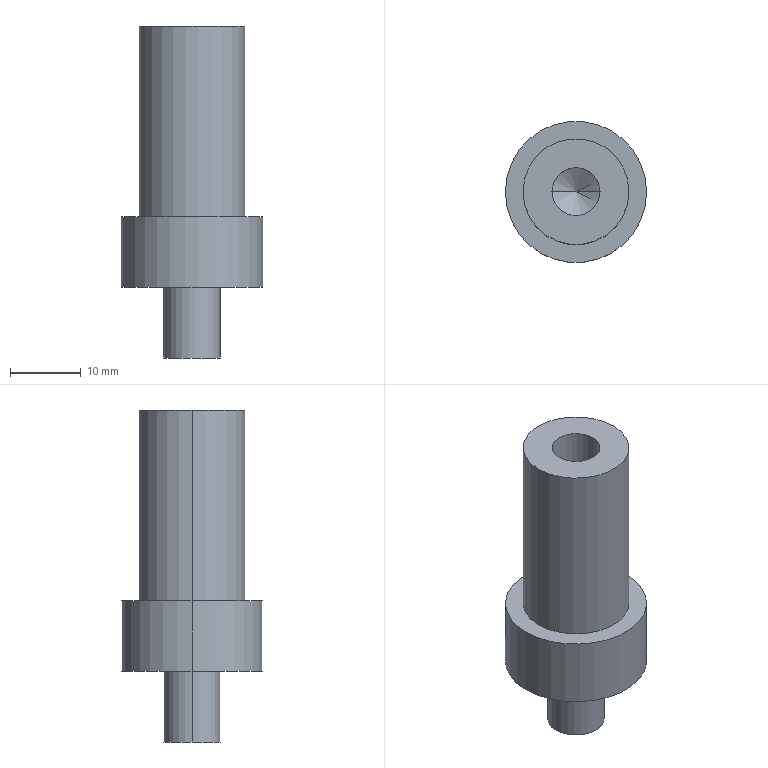Part | 1 solid | 14 faces | box 20 x 20 x 47 mm | volume 7810 mm3 | cylinder 8 | plane 4 | cone 2 | commonest cylinder face diameters 6.8 x2 8 x2 15 x2 20 x2
STEP:
#1=CARTESIAN_POINT('',(-4.,0.,-10.));
#2=VERTEX_POINT('',#1);
#3=CARTESIAN_POINT('',(4.,0.,-10.));
#4=VERTEX_POINT('',#3);
#5=CARTESIAN_POINT('',(0.,0.,-10.));
#6=DIRECTION('',(0.,0.,-1.));
#7=DIRECTION('',(-1.,0.,0.));
#8=AXIS2_PLACEMENT_3D('',#5,#6,#7);
#9=CIRCLE('',#8,4.);
#10=EDGE_CURVE('',#2,#4,#9,.T.);
#11=ORIENTED_EDGE('',*,*,#10,.F.);
#12=CARTESIAN_POINT('',(-4.,0.,0.));
#13=VERTEX_POINT('',#12);
#14=CARTESIAN_POINT('',(-4.,0.,-10.));
#15=DIRECTION('',(0.,0.,1.));
#16=VECTOR('',#15,1000.);
#17=LINE('',#14,#16);
#18=EDGE_CURVE('',#2,#13,#17,.T.);
#19=ORIENTED_EDGE('',*,*,#18,.T.);
#20=CARTESIAN_POINT('',(4.,0.,0.));
#21=VERTEX_POINT('',#20);
#22=CARTESIAN_POINT('',(0.,0.,0.));
#23=DIRECTION('',(0.,0.,-1.));
#24=DIRECTION('',(1.,0.,0.));
#25=AXIS2_PLACEMENT_3D('',#22,#23,#24);
#26=CIRCLE('',#25,4.);
#27=EDGE_CURVE('',#13,#21,#26,.T.);
#28=ORIENTED_EDGE('',*,*,#27,.T.);
#29=CARTESIAN_POINT('',(4.,0.,-10.));
#30=DIRECTION('',(0.,0.,1.));
#31=VECTOR('',#30,1000.);
#32=LINE('',#29,#31);
#33=EDGE_CURVE('',#4,#21,#32,.T.);
#34=ORIENTED_EDGE('',*,*,#33,.F.);
#35=EDGE_LOOP('',(#11,#19,#28,#34));
#36=FACE_OUTER_BOUND('',#35,.T.);
#37=CARTESIAN_POINT('',(0.,0.,-10.));
#38=DIRECTION('',(0.,0.,1.));
#39=DIRECTION('',(1.,0.,0.));
#40=AXIS2_PLACEMENT_3D('',#37,#38,#39);
#41=CYLINDRICAL_SURFACE('',#40,4.);
#42=ADVANCED_FACE('',(#36),#41,.T.);
#43=CARTESIAN_POINT('',(-3.4,0.,21.));
#44=VERTEX_POINT('',#43);
#45=CARTESIAN_POINT('',(3.4,0.,21.));
#46=VERTEX_POINT('',#45);
#47=CARTESIAN_POINT('',(0.,0.,21.));
#48=DIRECTION('',(0.,0.,1.));
#49=DIRECTION('',(1.,0.,0.));
#50=AXIS2_PLACEMENT_3D('',#47,#48,#49);
#51=CIRCLE('',#50,3.4);
#52=EDGE_CURVE('',#44,#46,#51,.T.);
#53=ORIENTED_EDGE('',*,*,#52,.F.);
#54=CARTESIAN_POINT('',(-3.4,0.,37.));
#55=VERTEX_POINT('',#54);
#56=CARTESIAN_POINT('',(-3.4,0.,37.));
#57=DIRECTION('',(0.,0.,1.));
#58=VECTOR('',#57,1000.);
#59=LINE('',#56,#58);
#60=EDGE_CURVE('',#44,#55,#59,.T.);
#61=ORIENTED_EDGE('',*,*,#60,.T.);
#62=CARTESIAN_POINT('',(3.4,0.,37.));
#63=VERTEX_POINT('',#62);
#64=CARTESIAN_POINT('',(0.,0.,37.));
#65=DIRECTION('',(0.,0.,1.));
#66=DIRECTION('',(1.,0.,0.));
#67=AXIS2_PLACEMENT_3D('',#64,#65,#66);
#68=CIRCLE('',#67,3.4);
#69=EDGE_CURVE('',#55,#63,#68,.T.);
#70=ORIENTED_EDGE('',*,*,#69,.T.);
#71=CARTESIAN_POINT('',(3.4,0.,37.));
#72=DIRECTION('',(0.,0.,1.));
#73=VECTOR('',#72,1000.);
#74=LINE('',#71,#73);
#75=EDGE_CURVE('',#46,#63,#74,.T.);
#76=ORIENTED_EDGE('',*,*,#75,.F.);
#77=EDGE_LOOP('',(#53,#61,#70,#76));
#78=FACE_OUTER_BOUND('',#77,.T.);
#79=CARTESIAN_POINT('',(0.,0.,37.));
#80=DIRECTION('',(0.,0.,1.));
#81=DIRECTION('',(1.,0.,0.));
#82=AXIS2_PLACEMENT_3D('',#79,#80,#81);
#83=CYLINDRICAL_SURFACE('',#82,3.4);
#84=ADVANCED_FACE('',(#78),#83,.F.);
#85=CARTESIAN_POINT('',(0.,0.,18.957));
#86=VERTEX_POINT('',#85);
#87=CARTESIAN_POINT('',(3.4,0.,21.));
#88=DIRECTION('',(0.8572,0.,0.515));
#89=VECTOR('',#88,1000.);
#90=LINE('',#87,#89);
#91=EDGE_CURVE('',#86,#46,#90,.T.);
#92=ORIENTED_EDGE('',*,*,#91,.F.);
#93=CARTESIAN_POINT('',(-3.4,0.,21.));
#94=DIRECTION('',(-0.8572,0.,0.515));
#95=VECTOR('',#94,1000.);
#96=LINE('',#93,#95);
#97=EDGE_CURVE('',#86,#44,#96,.T.);
#98=ORIENTED_EDGE('',*,*,#97,.T.);
#99=ORIENTED_EDGE('',*,*,#52,.T.);
#100=EDGE_LOOP('',(#92,#98,#99));
#101=FACE_OUTER_BOUND('',#100,.T.);
#102=CARTESIAN_POINT('',(0.,0.,21.));
#103=DIRECTION('',(0.,0.,1.));
#104=DIRECTION('',(1.,0.,0.));
#105=AXIS2_PLACEMENT_3D('',#102,#103,#104);
#106=CONICAL_SURFACE('',#105,3.4,1.03);
#107=ADVANCED_FACE('',(#101),#106,.F.);
#108=CARTESIAN_POINT('',(7.5,0.,37.));
#109=VERTEX_POINT('',#108);
#110=CARTESIAN_POINT('',(-7.5,0.,37.));
#111=VERTEX_POINT('',#110);
#112=CARTESIAN_POINT('',(0.,0.,37.));
#113=DIRECTION('',(0.,0.,1.));
#114=DIRECTION('',(1.,0.,0.));
#115=AXIS2_PLACEMENT_3D('',#112,#113,#114);
#116=CIRCLE('',#115,7.5);
#117=EDGE_CURVE('',#109,#111,#116,.T.);
#118=ORIENTED_EDGE('',*,*,#117,.F.);
#119=CARTESIAN_POINT('',(7.5,0.,10.));
#120=VERTEX_POINT('',#119);
#121=CARTESIAN_POINT('',(7.5,0.,37.));
#122=DIRECTION('',(0.,0.,-1.));
#123=VECTOR('',#122,1000.);
#124=LINE('',#121,#123);
#125=EDGE_CURVE('',#109,#120,#124,.T.);
#126=ORIENTED_EDGE('',*,*,#125,.T.);
#127=CARTESIAN_POINT('',(-7.5,0.,10.));
#128=VERTEX_POINT('',#127);
#129=CARTESIAN_POINT('',(0.,0.,10.));
#130=DIRECTION('',(0.,0.,1.));
#131=DIRECTION('',(1.,0.,0.));
#132=AXIS2_PLACEMENT_3D('',#129,#130,#131);
#133=CIRCLE('',#132,7.5);
#134=EDGE_CURVE('',#120,#128,#133,.T.);
#135=ORIENTED_EDGE('',*,*,#134,.T.);
#136=CARTESIAN_POINT('',(-7.5,0.,37.));
#137=DIRECTION('',(0.,0.,-1.));
#138=VECTOR('',#137,1000.);
#139=LINE('',#136,#138);
#140=EDGE_CURVE('',#111,#128,#139,.T.);
#141=ORIENTED_EDGE('',*,*,#140,.F.);
#142=EDGE_LOOP('',(#118,#126,#135,#141));
#143=FACE_OUTER_BOUND('',#142,.T.);
#144=CARTESIAN_POINT('',(0.,0.,37.));
#145=DIRECTION('',(0.,0.,-1.));
#146=DIRECTION('',(-1.,0.,0.));
#147=AXIS2_PLACEMENT_3D('',#144,#145,#146);
#148=CYLINDRICAL_SURFACE('',#147,7.5);
#149=ADVANCED_FACE('',(#143),#148,.T.);
#150=CARTESIAN_POINT('',(10.,0.,10.));
#151=VERTEX_POINT('',#150);
#152=CARTESIAN_POINT('',(-10.,0.,10.));
#153=VERTEX_POINT('',#152);
#154=CARTESIAN_POINT('',(0.,0.,10.));
#155=DIRECTION('',(0.,0.,1.));
#156=DIRECTION('',(1.,0.,0.));
#157=AXIS2_PLACEMENT_3D('',#154,#155,#156);
#158=CIRCLE('',#157,10.);
#159=EDGE_CURVE('',#151,#153,#158,.T.);
#160=ORIENTED_EDGE('',*,*,#159,.F.);
#161=CARTESIAN_POINT('',(10.,0.,0.));
#162=VERTEX_POINT('',#161);
#163=CARTESIAN_POINT('',(10.,0.,10.));
#164=DIRECTION('',(0.,0.,-1.));
#165=VECTOR('',#164,1000.);
#166=LINE('',#163,#165);
#167=EDGE_CURVE('',#151,#162,#166,.T.);
#168=ORIENTED_EDGE('',*,*,#167,.T.);
#169=CARTESIAN_POINT('',(-10.,0.,0.));
#170=VERTEX_POINT('',#169);
#171=CARTESIAN_POINT('',(0.,0.,0.));
#172=DIRECTION('',(0.,0.,1.));
#173=DIRECTION('',(1.,0.,0.));
#174=AXIS2_PLACEMENT_3D('',#171,#172,#173);
#175=CIRCLE('',#174,10.);
#176=EDGE_CURVE('',#162,#170,#175,.T.);
#177=ORIENTED_EDGE('',*,*,#176,.T.);
#178=CARTESIAN_POINT('',(-10.,0.,10.));
#179=DIRECTION('',(0.,0.,-1.));
#180=VECTOR('',#179,1000.);
#181=LINE('',#178,#180);
#182=EDGE_CURVE('',#153,#170,#181,.T.);
#183=ORIENTED_EDGE('',*,*,#182,.F.);
#184=EDGE_LOOP('',(#160,#168,#177,#183));
#185=FACE_OUTER_BOUND('',#184,.T.);
#186=CARTESIAN_POINT('',(0.,0.,10.));
#187=DIRECTION('',(0.,0.,-1.));
#188=DIRECTION('',(-1.,0.,0.));
#189=AXIS2_PLACEMENT_3D('',#186,#187,#188);
#190=CYLINDRICAL_SURFACE('',#189,10.);
#191=ADVANCED_FACE('',(#185),#190,.T.);
#192=CARTESIAN_POINT('',(0.,0.,0.));
#193=DIRECTION('',(0.,0.,1.));
#194=DIRECTION('',(1.,0.,0.));
#195=AXIS2_PLACEMENT_3D('',#192,#193,#194);
#196=CIRCLE('',#195,10.);
#197=EDGE_CURVE('',#170,#162,#196,.T.);
#198=ORIENTED_EDGE('',*,*,#197,.F.);
#199=ORIENTED_EDGE('',*,*,#176,.F.);
#200=EDGE_LOOP('',(#198,#199));
#201=FACE_OUTER_BOUND('',#200,.T.);
#202=CARTESIAN_POINT('',(0.,0.,0.));
#203=DIRECTION('',(0.,0.,-1.));
#204=DIRECTION('',(1.,0.,0.));
#205=AXIS2_PLACEMENT_3D('',#202,#203,#204);
#206=CIRCLE('',#205,4.);
#207=EDGE_CURVE('',#21,#13,#206,.T.);
#208=ORIENTED_EDGE('',*,*,#207,.F.);
#209=ORIENTED_EDGE('',*,*,#27,.F.);
#210=EDGE_LOOP('',(#208,#209));
#211=FACE_BOUND('',#210,.T.);
#212=CARTESIAN_POINT('',(0.,0.,0.));
#213=DIRECTION('',(0.,0.,1.));
#214=DIRECTION('',(1.,0.,0.));
#215=AXIS2_PLACEMENT_3D('',#212,#213,#214);
#216=PLANE('',#215);
#217=ADVANCED_FACE('',(#201,#211),#216,.F.);
#218=CARTESIAN_POINT('',(0.,0.,10.));
#219=DIRECTION('',(0.,0.,1.));
#220=DIRECTION('',(1.,0.,0.));
#221=AXIS2_PLACEMENT_3D('',#218,#219,#220);
#222=CIRCLE('',#221,10.);
#223=EDGE_CURVE('',#153,#151,#222,.T.);
#224=ORIENTED_EDGE('',*,*,#223,.T.);
#225=ORIENTED_EDGE('',*,*,#159,.T.);
#226=EDGE_LOOP('',(#224,#225));
#227=FACE_OUTER_BOUND('',#226,.T.);
#228=CARTESIAN_POINT('',(0.,0.,10.));
#229=DIRECTION('',(0.,0.,1.));
#230=DIRECTION('',(1.,0.,0.));
#231=AXIS2_PLACEMENT_3D('',#228,#229,#230);
#232=CIRCLE('',#231,7.5);
#233=EDGE_CURVE('',#128,#120,#232,.T.);
#234=ORIENTED_EDGE('',*,*,#233,.F.);
#235=ORIENTED_EDGE('',*,*,#134,.F.);
#236=EDGE_LOOP('',(#234,#235));
#237=FACE_BOUND('',#236,.T.);
#238=CARTESIAN_POINT('',(0.,0.,10.));
#239=DIRECTION('',(0.,0.,1.));
#240=DIRECTION('',(1.,0.,0.));
#241=AXIS2_PLACEMENT_3D('',#238,#239,#240);
#242=PLANE('',#241);
#243=ADVANCED_FACE('',(#227,#237),#242,.T.);
#244=ORIENTED_EDGE('',*,*,#167,.F.);
#245=ORIENTED_EDGE('',*,*,#223,.F.);
#246=ORIENTED_EDGE('',*,*,#182,.T.);
#247=ORIENTED_EDGE('',*,*,#197,.T.);
#248=EDGE_LOOP('',(#244,#245,#246,#247));
#249=FACE_OUTER_BOUND('',#248,.T.);
#250=CARTESIAN_POINT('',(0.,0.,10.));
#251=DIRECTION('',(0.,0.,-1.));
#252=DIRECTION('',(-1.,0.,0.));
#253=AXIS2_PLACEMENT_3D('',#250,#251,#252);
#254=CYLINDRICAL_SURFACE('',#253,10.);
#255=ADVANCED_FACE('',(#249),#254,.T.);
#256=ORIENTED_EDGE('',*,*,#125,.F.);
#257=CARTESIAN_POINT('',(0.,0.,37.));
#258=DIRECTION('',(0.,0.,1.));
#259=DIRECTION('',(1.,0.,0.));
#260=AXIS2_PLACEMENT_3D('',#257,#258,#259);
#261=CIRCLE('',#260,7.5);
#262=EDGE_CURVE('',#111,#109,#261,.T.);
#263=ORIENTED_EDGE('',*,*,#262,.F.);
#264=ORIENTED_EDGE('',*,*,#140,.T.);
#265=ORIENTED_EDGE('',*,*,#233,.T.);
#266=EDGE_LOOP('',(#256,#263,#264,#265));
#267=FACE_OUTER_BOUND('',#266,.T.);
#268=CARTESIAN_POINT('',(0.,0.,37.));
#269=DIRECTION('',(0.,0.,-1.));
#270=DIRECTION('',(-1.,0.,0.));
#271=AXIS2_PLACEMENT_3D('',#268,#269,#270);
#272=CYLINDRICAL_SURFACE('',#271,7.5);
#273=ADVANCED_FACE('',(#267),#272,.T.);
#274=CARTESIAN_POINT('',(0.,0.,37.));
#275=DIRECTION('',(0.,0.,1.));
#276=DIRECTION('',(1.,0.,0.));
#277=AXIS2_PLACEMENT_3D('',#274,#275,#276);
#278=CIRCLE('',#277,3.4);
#279=EDGE_CURVE('',#63,#55,#278,.T.);
#280=ORIENTED_EDGE('',*,*,#279,.F.);
#281=ORIENTED_EDGE('',*,*,#69,.F.);
#282=EDGE_LOOP('',(#280,#281));
#283=FACE_BOUND('',#282,.T.);
#284=ORIENTED_EDGE('',*,*,#262,.T.);
#285=ORIENTED_EDGE('',*,*,#117,.T.);
#286=EDGE_LOOP('',(#284,#285));
#287=FACE_OUTER_BOUND('',#286,.T.);
#288=CARTESIAN_POINT('',(0.,0.,37.));
#289=DIRECTION('',(0.,0.,1.));
#290=DIRECTION('',(1.,0.,0.));
#291=AXIS2_PLACEMENT_3D('',#288,#289,#290);
#292=PLANE('',#291);
#293=ADVANCED_FACE('',(#283,#287),#292,.T.);
#294=ORIENTED_EDGE('',*,*,#97,.F.);
#295=ORIENTED_EDGE('',*,*,#91,.T.);
#296=CARTESIAN_POINT('',(0.,0.,21.));
#297=DIRECTION('',(0.,0.,1.));
#298=DIRECTION('',(1.,0.,0.));
#299=AXIS2_PLACEMENT_3D('',#296,#297,#298);
#300=CIRCLE('',#299,3.4);
#301=EDGE_CURVE('',#46,#44,#300,.T.);
#302=ORIENTED_EDGE('',*,*,#301,.T.);
#303=EDGE_LOOP('',(#294,#295,#302));
#304=FACE_OUTER_BOUND('',#303,.T.);
#305=CARTESIAN_POINT('',(0.,0.,21.));
#306=DIRECTION('',(0.,0.,1.));
#307=DIRECTION('',(1.,0.,0.));
#308=AXIS2_PLACEMENT_3D('',#305,#306,#307);
#309=CONICAL_SURFACE('',#308,3.4,1.03);
#310=ADVANCED_FACE('',(#304),#309,.F.);
#311=ORIENTED_EDGE('',*,*,#60,.F.);
#312=ORIENTED_EDGE('',*,*,#301,.F.);
#313=ORIENTED_EDGE('',*,*,#75,.T.);
#314=ORIENTED_EDGE('',*,*,#279,.T.);
#315=EDGE_LOOP('',(#311,#312,#313,#314));
#316=FACE_OUTER_BOUND('',#315,.T.);
#317=CARTESIAN_POINT('',(0.,0.,37.));
#318=DIRECTION('',(0.,0.,1.));
#319=DIRECTION('',(1.,0.,0.));
#320=AXIS2_PLACEMENT_3D('',#317,#318,#319);
#321=CYLINDRICAL_SURFACE('',#320,3.4);
#322=ADVANCED_FACE('',(#316),#321,.F.);
#323=ORIENTED_EDGE('',*,*,#18,.F.);
#324=CARTESIAN_POINT('',(0.,0.,-10.));
#325=DIRECTION('',(0.,0.,-1.));
#326=DIRECTION('',(-1.,0.,0.));
#327=AXIS2_PLACEMENT_3D('',#324,#325,#326);
#328=CIRCLE('',#327,4.);
#329=EDGE_CURVE('',#4,#2,#328,.T.);
#330=ORIENTED_EDGE('',*,*,#329,.F.);
#331=ORIENTED_EDGE('',*,*,#33,.T.);
#332=ORIENTED_EDGE('',*,*,#207,.T.);
#333=EDGE_LOOP('',(#323,#330,#331,#332));
#334=FACE_OUTER_BOUND('',#333,.T.);
#335=CARTESIAN_POINT('',(0.,0.,-10.));
#336=DIRECTION('',(0.,0.,1.));
#337=DIRECTION('',(1.,0.,0.));
#338=AXIS2_PLACEMENT_3D('',#335,#336,#337);
#339=CYLINDRICAL_SURFACE('',#338,4.);
#340=ADVANCED_FACE('',(#334),#339,.T.);
#341=ORIENTED_EDGE('',*,*,#329,.T.);
#342=ORIENTED_EDGE('',*,*,#10,.T.);
#343=EDGE_LOOP('',(#341,#342));
#344=FACE_OUTER_BOUND('',#343,.T.);
#345=CARTESIAN_POINT('',(0.,0.,-10.));
#346=DIRECTION('',(0.,0.,-1.));
#347=DIRECTION('',(-1.,0.,0.));
#348=AXIS2_PLACEMENT_3D('',#345,#346,#347);
#349=PLANE('',#348);
#350=ADVANCED_FACE('',(#344),#349,.T.);
#351=CLOSED_SHELL('',(#42,#84,#107,#149,#191,#217,#243,#255,#273,#293,#310,#322,#340,#350));
#352=MANIFOLD_SOLID_BREP('',#351);
#353=CARTESIAN_POINT('',(0.,0.,0.));
#354=DIRECTION('',(0.,0.,1.));
#355=DIRECTION('',(1.,0.,0.));
#356=AXIS2_PLACEMENT_3D('',#353,#354,#355);
#357=(LENGTH_UNIT()NAMED_UNIT(*)SI_UNIT(.MILLI.,.METRE.));
#358=UNCERTAINTY_MEASURE_WITH_UNIT(LENGTH_MEASURE(0.00001),#357,'','');
#359=(NAMED_UNIT(*)PLANE_ANGLE_UNIT()SI_UNIT($,.RADIAN.));
#360=(NAMED_UNIT(*)SI_UNIT($,.STERADIAN.)SOLID_ANGLE_UNIT());
#361=(GEOMETRIC_REPRESENTATION_CONTEXT(3)GLOBAL_UNCERTAINTY_ASSIGNED_CONTEXT((#358))GLOBAL_UNIT_ASSIGNED_CONTEXT((#357,#359,#360))REPRESENTATION_CONTEXT('',''));
#362=ADVANCED_BREP_SHAPE_REPRESENTATION('',(#352,#356),#361);